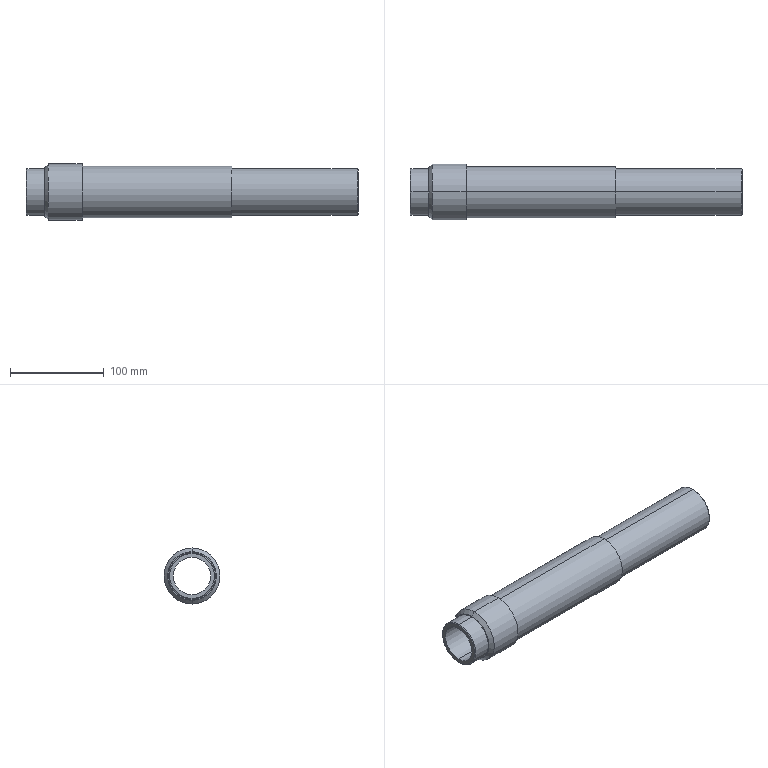Part | SolidWorks | features Chamfer 1, Fillet 1, Revolution 1 | 1 solid | 23 faces | box 355 x 60 x 60 mm | volume 349894 mm3 | cylinder 10 | plane 5 | cone 4 | torus 4 | commonest cylinder face diameters 50 x4 40 x2 55 x2 60 x2
STEP:
#1=CARTESIAN_POINT('',(354.,0.,20.));
#2=VERTEX_POINT('',#1);
#3=CARTESIAN_POINT('',(354.,0.,-20.));
#4=VERTEX_POINT('',#3);
#5=CARTESIAN_POINT('',(354.,0.,0.));
#6=DIRECTION('',(1.,0.,0.));
#7=DIRECTION('',(0.,0.,1.));
#8=AXIS2_PLACEMENT_3D('',#5,#6,#7);
#9=CIRCLE('',#8,20.);
#10=EDGE_CURVE('',#2,#4,#9,.T.);
#11=ORIENTED_EDGE('',*,*,#10,.F.);
#12=CARTESIAN_POINT('',(355.,0.,21.));
#13=VERTEX_POINT('',#12);
#14=CARTESIAN_POINT('',(355.,0.,21.));
#15=DIRECTION('',(0.7071,0.,0.7071));
#16=VECTOR('',#15,1000.);
#17=LINE('',#14,#16);
#18=EDGE_CURVE('',#2,#13,#17,.T.);
#19=ORIENTED_EDGE('',*,*,#18,.T.);
#20=CARTESIAN_POINT('',(355.,0.,-21.));
#21=VERTEX_POINT('',#20);
#22=CARTESIAN_POINT('',(355.,0.,0.));
#23=DIRECTION('',(-1.,0.,0.));
#24=DIRECTION('',(0.,0.,1.));
#25=AXIS2_PLACEMENT_3D('',#22,#23,#24);
#26=CIRCLE('',#25,21.);
#27=EDGE_CURVE('',#21,#13,#26,.T.);
#28=ORIENTED_EDGE('',*,*,#27,.F.);
#29=CARTESIAN_POINT('',(355.,0.,-21.));
#30=DIRECTION('',(0.7071,0.,-0.7071));
#31=VECTOR('',#30,1000.);
#32=LINE('',#29,#31);
#33=EDGE_CURVE('',#4,#21,#32,.T.);
#34=ORIENTED_EDGE('',*,*,#33,.F.);
#35=EDGE_LOOP('',(#11,#19,#28,#34));
#36=FACE_OUTER_BOUND('',#35,.T.);
#37=CARTESIAN_POINT('',(355.,0.,0.));
#38=DIRECTION('',(1.,0.,0.));
#39=DIRECTION('',(0.,0.,-1.));
#40=AXIS2_PLACEMENT_3D('',#37,#38,#39);
#41=CONICAL_SURFACE('',#40,21.,0.7854);
#42=ADVANCED_FACE('',(#36),#41,.F.);
#43=CARTESIAN_POINT('',(1.,0.,-25.));
#44=VERTEX_POINT('',#43);
#45=CARTESIAN_POINT('',(1.,0.,25.));
#46=VERTEX_POINT('',#45);
#47=CARTESIAN_POINT('',(1.,0.,0.));
#48=DIRECTION('',(1.,0.,0.));
#49=DIRECTION('',(0.,0.,1.));
#50=AXIS2_PLACEMENT_3D('',#47,#48,#49);
#51=CIRCLE('',#50,25.);
#52=EDGE_CURVE('',#44,#46,#51,.T.);
#53=ORIENTED_EDGE('',*,*,#52,.F.);
#54=CARTESIAN_POINT('',(0.,0.,-24.));
#55=VERTEX_POINT('',#54);
#56=CARTESIAN_POINT('',(1.,0.,-24.));
#57=DIRECTION('',(0.,1.,0.));
#58=DIRECTION('',(0.,0.,1.));
#59=AXIS2_PLACEMENT_3D('',#56,#57,#58);
#60=CIRCLE('',#59,1.);
#61=EDGE_CURVE('',#44,#55,#60,.T.);
#62=ORIENTED_EDGE('',*,*,#61,.T.);
#63=CARTESIAN_POINT('',(0.,0.,24.));
#64=VERTEX_POINT('',#63);
#65=CARTESIAN_POINT('',(0.,0.,0.));
#66=DIRECTION('',(-1.,0.,0.));
#67=DIRECTION('',(0.,0.,1.));
#68=AXIS2_PLACEMENT_3D('',#65,#66,#67);
#69=CIRCLE('',#68,24.);
#70=EDGE_CURVE('',#64,#55,#69,.T.);
#71=ORIENTED_EDGE('',*,*,#70,.F.);
#72=CARTESIAN_POINT('',(1.,0.,24.));
#73=DIRECTION('',(0.,-1.,0.));
#74=DIRECTION('',(0.,0.,-1.));
#75=AXIS2_PLACEMENT_3D('',#72,#73,#74);
#76=CIRCLE('',#75,1.);
#77=EDGE_CURVE('',#46,#64,#76,.T.);
#78=ORIENTED_EDGE('',*,*,#77,.F.);
#79=EDGE_LOOP('',(#53,#62,#71,#78));
#80=FACE_OUTER_BOUND('',#79,.T.);
#81=CARTESIAN_POINT('',(1.,0.,0.));
#82=DIRECTION('',(-1.,0.,0.));
#83=DIRECTION('',(0.,0.,1.));
#84=AXIS2_PLACEMENT_3D('',#81,#82,#83);
#85=TOROIDAL_SURFACE('',#84,24.,1.);
#86=ADVANCED_FACE('',(#80),#85,.T.);
#87=CARTESIAN_POINT('',(355.,0.,-24.));
#88=VERTEX_POINT('',#87);
#89=CARTESIAN_POINT('',(355.,0.,24.));
#90=VERTEX_POINT('',#89);
#91=CARTESIAN_POINT('',(355.,0.,0.));
#92=DIRECTION('',(1.,0.,0.));
#93=DIRECTION('',(0.,0.,1.));
#94=AXIS2_PLACEMENT_3D('',#91,#92,#93);
#95=CIRCLE('',#94,24.);
#96=EDGE_CURVE('',#88,#90,#95,.T.);
#97=ORIENTED_EDGE('',*,*,#96,.F.);
#98=CARTESIAN_POINT('',(354.,0.,-25.));
#99=VERTEX_POINT('',#98);
#100=CARTESIAN_POINT('',(354.,0.,-24.));
#101=DIRECTION('',(0.,1.,0.));
#102=DIRECTION('',(0.,0.,1.));
#103=AXIS2_PLACEMENT_3D('',#100,#101,#102);
#104=CIRCLE('',#103,1.);
#105=EDGE_CURVE('',#88,#99,#104,.T.);
#106=ORIENTED_EDGE('',*,*,#105,.T.);
#107=CARTESIAN_POINT('',(354.,0.,25.));
#108=VERTEX_POINT('',#107);
#109=CARTESIAN_POINT('',(354.,0.,0.));
#110=DIRECTION('',(-1.,0.,0.));
#111=DIRECTION('',(0.,0.,1.));
#112=AXIS2_PLACEMENT_3D('',#109,#110,#111);
#113=CIRCLE('',#112,25.);
#114=EDGE_CURVE('',#108,#99,#113,.T.);
#115=ORIENTED_EDGE('',*,*,#114,.F.);
#116=CARTESIAN_POINT('',(354.,0.,24.));
#117=DIRECTION('',(0.,-1.,0.));
#118=DIRECTION('',(0.,0.,-1.));
#119=AXIS2_PLACEMENT_3D('',#116,#117,#118);
#120=CIRCLE('',#119,1.);
#121=EDGE_CURVE('',#90,#108,#120,.T.);
#122=ORIENTED_EDGE('',*,*,#121,.F.);
#123=EDGE_LOOP('',(#97,#106,#115,#122));
#124=FACE_OUTER_BOUND('',#123,.T.);
#125=CARTESIAN_POINT('',(354.,0.,0.));
#126=DIRECTION('',(-1.,0.,0.));
#127=DIRECTION('',(0.,0.,1.));
#128=AXIS2_PLACEMENT_3D('',#125,#126,#127);
#129=TOROIDAL_SURFACE('',#128,24.,1.);
#130=ADVANCED_FACE('',(#124),#129,.T.);
#131=CARTESIAN_POINT('',(20.,0.,26.));
#132=VERTEX_POINT('',#131);
#133=CARTESIAN_POINT('',(20.,0.,-26.));
#134=VERTEX_POINT('',#133);
#135=CARTESIAN_POINT('',(20.,0.,0.));
#136=DIRECTION('',(-1.,0.,0.));
#137=DIRECTION('',(0.,0.,1.));
#138=AXIS2_PLACEMENT_3D('',#135,#136,#137);
#139=CIRCLE('',#138,26.);
#140=EDGE_CURVE('',#132,#134,#139,.T.);
#141=ORIENTED_EDGE('',*,*,#140,.F.);
#142=CARTESIAN_POINT('',(24.,0.,30.));
#143=VERTEX_POINT('',#142);
#144=CARTESIAN_POINT('',(20.,0.,26.));
#145=DIRECTION('',(0.7071,0.,0.7071));
#146=VECTOR('',#145,1000.);
#147=LINE('',#144,#146);
#148=EDGE_CURVE('',#132,#143,#147,.T.);
#149=ORIENTED_EDGE('',*,*,#148,.T.);
#150=CARTESIAN_POINT('',(24.,0.,-30.));
#151=VERTEX_POINT('',#150);
#152=CARTESIAN_POINT('',(24.,0.,0.));
#153=DIRECTION('',(-1.,0.,0.));
#154=DIRECTION('',(0.,0.,1.));
#155=AXIS2_PLACEMENT_3D('',#152,#153,#154);
#156=CIRCLE('',#155,30.);
#157=EDGE_CURVE('',#143,#151,#156,.T.);
#158=ORIENTED_EDGE('',*,*,#157,.T.);
#159=CARTESIAN_POINT('',(20.,0.,-26.));
#160=DIRECTION('',(0.7071,0.,-0.7071));
#161=VECTOR('',#160,1000.);
#162=LINE('',#159,#161);
#163=EDGE_CURVE('',#134,#151,#162,.T.);
#164=ORIENTED_EDGE('',*,*,#163,.F.);
#165=EDGE_LOOP('',(#141,#149,#158,#164));
#166=FACE_OUTER_BOUND('',#165,.T.);
#167=CARTESIAN_POINT('',(20.,0.,0.));
#168=DIRECTION('',(1.,0.,0.));
#169=DIRECTION('',(0.,0.,-1.));
#170=AXIS2_PLACEMENT_3D('',#167,#168,#169);
#171=CONICAL_SURFACE('',#170,26.,0.7854);
#172=ADVANCED_FACE('',(#166),#171,.T.);
#173=CARTESIAN_POINT('',(60.,0.,30.));
#174=VERTEX_POINT('',#173);
#175=CARTESIAN_POINT('',(60.,0.,-30.));
#176=VERTEX_POINT('',#175);
#177=CARTESIAN_POINT('',(60.,0.,0.));
#178=DIRECTION('',(-1.,0.,0.));
#179=DIRECTION('',(0.,0.,1.));
#180=AXIS2_PLACEMENT_3D('',#177,#178,#179);
#181=CIRCLE('',#180,30.);
#182=EDGE_CURVE('',#174,#176,#181,.T.);
#183=ORIENTED_EDGE('',*,*,#182,.T.);
#184=CARTESIAN_POINT('',(20.,0.,-30.));
#185=DIRECTION('',(-1.,0.,0.));
#186=VECTOR('',#185,1000.);
#187=LINE('',#184,#186);
#188=EDGE_CURVE('',#176,#151,#187,.T.);
#189=ORIENTED_EDGE('',*,*,#188,.T.);
#190=ORIENTED_EDGE('',*,*,#157,.F.);
#191=CARTESIAN_POINT('',(20.,0.,30.));
#192=DIRECTION('',(-1.,0.,0.));
#193=VECTOR('',#192,1000.);
#194=LINE('',#191,#193);
#195=EDGE_CURVE('',#174,#143,#194,.T.);
#196=ORIENTED_EDGE('',*,*,#195,.F.);
#197=EDGE_LOOP('',(#183,#189,#190,#196));
#198=FACE_OUTER_BOUND('',#197,.T.);
#199=CARTESIAN_POINT('',(20.,0.,0.));
#200=DIRECTION('',(-1.,0.,0.));
#201=DIRECTION('',(0.,0.,1.));
#202=AXIS2_PLACEMENT_3D('',#199,#200,#201);
#203=CYLINDRICAL_SURFACE('',#202,30.);
#204=ADVANCED_FACE('',(#198),#203,.T.);
#205=CARTESIAN_POINT('',(220.,0.,27.5));
#206=VERTEX_POINT('',#205);
#207=CARTESIAN_POINT('',(220.,0.,-27.5));
#208=VERTEX_POINT('',#207);
#209=CARTESIAN_POINT('',(220.,0.,0.));
#210=DIRECTION('',(-1.,0.,0.));
#211=DIRECTION('',(0.,0.,1.));
#212=AXIS2_PLACEMENT_3D('',#209,#210,#211);
#213=CIRCLE('',#212,27.5);
#214=EDGE_CURVE('',#206,#208,#213,.T.);
#215=ORIENTED_EDGE('',*,*,#214,.T.);
#216=CARTESIAN_POINT('',(60.,0.,-27.5));
#217=VERTEX_POINT('',#216);
#218=CARTESIAN_POINT('',(20.,0.,-27.5));
#219=DIRECTION('',(-1.,0.,0.));
#220=VECTOR('',#219,1000.);
#221=LINE('',#218,#220);
#222=EDGE_CURVE('',#208,#217,#221,.T.);
#223=ORIENTED_EDGE('',*,*,#222,.T.);
#224=CARTESIAN_POINT('',(60.,0.,27.5));
#225=VERTEX_POINT('',#224);
#226=CARTESIAN_POINT('',(60.,0.,0.));
#227=DIRECTION('',(-1.,0.,0.));
#228=DIRECTION('',(0.,0.,1.));
#229=AXIS2_PLACEMENT_3D('',#226,#227,#228);
#230=CIRCLE('',#229,27.5);
#231=EDGE_CURVE('',#225,#217,#230,.T.);
#232=ORIENTED_EDGE('',*,*,#231,.F.);
#233=CARTESIAN_POINT('',(20.,0.,27.5));
#234=DIRECTION('',(-1.,0.,0.));
#235=VECTOR('',#234,1000.);
#236=LINE('',#233,#235);
#237=EDGE_CURVE('',#206,#225,#236,.T.);
#238=ORIENTED_EDGE('',*,*,#237,.F.);
#239=EDGE_LOOP('',(#215,#223,#232,#238));
#240=FACE_OUTER_BOUND('',#239,.T.);
#241=CARTESIAN_POINT('',(20.,0.,0.));
#242=DIRECTION('',(-1.,0.,0.));
#243=DIRECTION('',(0.,0.,1.));
#244=AXIS2_PLACEMENT_3D('',#241,#242,#243);
#245=CYLINDRICAL_SURFACE('',#244,27.5);
#246=ADVANCED_FACE('',(#240),#245,.T.);
#247=ORIENTED_EDGE('',*,*,#114,.T.);
#248=CARTESIAN_POINT('',(220.,0.,-25.));
#249=VERTEX_POINT('',#248);
#250=CARTESIAN_POINT('',(20.,0.,-25.));
#251=DIRECTION('',(-1.,0.,0.));
#252=VECTOR('',#251,1000.);
#253=LINE('',#250,#252);
#254=EDGE_CURVE('',#99,#249,#253,.T.);
#255=ORIENTED_EDGE('',*,*,#254,.T.);
#256=CARTESIAN_POINT('',(220.,0.,25.));
#257=VERTEX_POINT('',#256);
#258=CARTESIAN_POINT('',(220.,0.,0.));
#259=DIRECTION('',(-1.,0.,0.));
#260=DIRECTION('',(0.,0.,1.));
#261=AXIS2_PLACEMENT_3D('',#258,#259,#260);
#262=CIRCLE('',#261,25.);
#263=EDGE_CURVE('',#257,#249,#262,.T.);
#264=ORIENTED_EDGE('',*,*,#263,.F.);
#265=CARTESIAN_POINT('',(20.,0.,25.));
#266=DIRECTION('',(-1.,0.,0.));
#267=VECTOR('',#266,1000.);
#268=LINE('',#265,#267);
#269=EDGE_CURVE('',#108,#257,#268,.T.);
#270=ORIENTED_EDGE('',*,*,#269,.F.);
#271=EDGE_LOOP('',(#247,#255,#264,#270));
#272=FACE_OUTER_BOUND('',#271,.T.);
#273=CARTESIAN_POINT('',(20.,0.,0.));
#274=DIRECTION('',(-1.,0.,0.));
#275=DIRECTION('',(0.,0.,1.));
#276=AXIS2_PLACEMENT_3D('',#273,#274,#275);
#277=CYLINDRICAL_SURFACE('',#276,25.);
#278=ADVANCED_FACE('',(#272),#277,.T.);
#279=ORIENTED_EDGE('',*,*,#10,.T.);
#280=CARTESIAN_POINT('',(0.,0.,-20.));
#281=VERTEX_POINT('',#280);
#282=CARTESIAN_POINT('',(20.,0.,-20.));
#283=DIRECTION('',(-1.,0.,0.));
#284=VECTOR('',#283,1000.);
#285=LINE('',#282,#284);
#286=EDGE_CURVE('',#4,#281,#285,.T.);
#287=ORIENTED_EDGE('',*,*,#286,.T.);
#288=CARTESIAN_POINT('',(0.,0.,20.));
#289=VERTEX_POINT('',#288);
#290=CARTESIAN_POINT('',(0.,0.,0.));
#291=DIRECTION('',(-1.,0.,0.));
#292=DIRECTION('',(0.,0.,1.));
#293=AXIS2_PLACEMENT_3D('',#290,#291,#292);
#294=CIRCLE('',#293,20.);
#295=EDGE_CURVE('',#281,#289,#294,.T.);
#296=ORIENTED_EDGE('',*,*,#295,.T.);
#297=CARTESIAN_POINT('',(20.,0.,20.));
#298=DIRECTION('',(-1.,0.,0.));
#299=VECTOR('',#298,1000.);
#300=LINE('',#297,#299);
#301=EDGE_CURVE('',#2,#289,#300,.T.);
#302=ORIENTED_EDGE('',*,*,#301,.F.);
#303=EDGE_LOOP('',(#279,#287,#296,#302));
#304=FACE_OUTER_BOUND('',#303,.T.);
#305=CARTESIAN_POINT('',(20.,0.,0.));
#306=DIRECTION('',(-1.,0.,0.));
#307=DIRECTION('',(0.,0.,1.));
#308=AXIS2_PLACEMENT_3D('',#305,#306,#307);
#309=CYLINDRICAL_SURFACE('',#308,20.);
#310=ADVANCED_FACE('',(#304),#309,.F.);
#311=CARTESIAN_POINT('',(20.,0.,25.));
#312=VERTEX_POINT('',#311);
#313=CARTESIAN_POINT('',(20.,0.,-25.));
#314=VERTEX_POINT('',#313);
#315=CARTESIAN_POINT('',(20.,0.,0.));
#316=DIRECTION('',(-1.,0.,0.));
#317=DIRECTION('',(0.,0.,1.));
#318=AXIS2_PLACEMENT_3D('',#315,#316,#317);
#319=CIRCLE('',#318,25.);
#320=EDGE_CURVE('',#312,#314,#319,.T.);
#321=ORIENTED_EDGE('',*,*,#320,.T.);
#322=CARTESIAN_POINT('',(20.,0.,-25.));
#323=DIRECTION('',(-1.,0.,0.));
#324=VECTOR('',#323,1000.);
#325=LINE('',#322,#324);
#326=EDGE_CURVE('',#314,#44,#325,.T.);
#327=ORIENTED_EDGE('',*,*,#326,.T.);
#328=ORIENTED_EDGE('',*,*,#52,.T.);
#329=CARTESIAN_POINT('',(20.,0.,25.));
#330=DIRECTION('',(-1.,0.,0.));
#331=VECTOR('',#330,1000.);
#332=LINE('',#329,#331);
#333=EDGE_CURVE('',#312,#46,#332,.T.);
#334=ORIENTED_EDGE('',*,*,#333,.F.);
#335=EDGE_LOOP('',(#321,#327,#328,#334));
#336=FACE_OUTER_BOUND('',#335,.T.);
#337=CARTESIAN_POINT('',(20.,0.,0.));
#338=DIRECTION('',(-1.,0.,0.));
#339=DIRECTION('',(0.,0.,1.));
#340=AXIS2_PLACEMENT_3D('',#337,#338,#339);
#341=CYLINDRICAL_SURFACE('',#340,25.);
#342=ADVANCED_FACE('',(#336),#341,.T.);
#343=ORIENTED_EDGE('',*,*,#326,.F.);
#344=CARTESIAN_POINT('',(20.,0.,0.));
#345=DIRECTION('',(-1.,0.,0.));
#346=DIRECTION('',(0.,0.,1.));
#347=AXIS2_PLACEMENT_3D('',#344,#345,#346);
#348=CIRCLE('',#347,25.);
#349=EDGE_CURVE('',#314,#312,#348,.T.);
#350=ORIENTED_EDGE('',*,*,#349,.T.);
#351=ORIENTED_EDGE('',*,*,#333,.T.);
#352=CARTESIAN_POINT('',(1.,0.,0.));
#353=DIRECTION('',(1.,0.,0.));
#354=DIRECTION('',(0.,0.,1.));
#355=AXIS2_PLACEMENT_3D('',#352,#353,#354);
#356=CIRCLE('',#355,25.);
#357=EDGE_CURVE('',#46,#44,#356,.T.);
#358=ORIENTED_EDGE('',*,*,#357,.T.);
#359=EDGE_LOOP('',(#343,#350,#351,#358));
#360=FACE_OUTER_BOUND('',#359,.T.);
#361=CARTESIAN_POINT('',(20.,0.,0.));
#362=DIRECTION('',(-1.,0.,0.));
#363=DIRECTION('',(0.,0.,1.));
#364=AXIS2_PLACEMENT_3D('',#361,#362,#363);
#365=CYLINDRICAL_SURFACE('',#364,25.);
#366=ADVANCED_FACE('',(#360),#365,.T.);
#367=ORIENTED_EDGE('',*,*,#70,.T.);
#368=CARTESIAN_POINT('',(0.,0.,0.));
#369=DIRECTION('',(-1.,0.,0.));
#370=DIRECTION('',(0.,0.,1.));
#371=AXIS2_PLACEMENT_3D('',#368,#369,#370);
#372=CIRCLE('',#371,24.);
#373=EDGE_CURVE('',#55,#64,#372,.T.);
#374=ORIENTED_EDGE('',*,*,#373,.T.);
#375=EDGE_LOOP('',(#367,#374));
#376=FACE_OUTER_BOUND('',#375,.T.);
#377=CARTESIAN_POINT('',(0.,0.,0.));
#378=DIRECTION('',(-1.,0.,0.));
#379=DIRECTION('',(0.,0.,1.));
#380=AXIS2_PLACEMENT_3D('',#377,#378,#379);
#381=CIRCLE('',#380,20.);
#382=EDGE_CURVE('',#289,#281,#381,.T.);
#383=ORIENTED_EDGE('',*,*,#382,.F.);
#384=ORIENTED_EDGE('',*,*,#295,.F.);
#385=EDGE_LOOP('',(#383,#384));
#386=FACE_BOUND('',#385,.T.);
#387=CARTESIAN_POINT('',(0.,0.,0.));
#388=DIRECTION('',(-1.,0.,0.));
#389=DIRECTION('',(0.,0.,1.));
#390=AXIS2_PLACEMENT_3D('',#387,#388,#389);
#391=PLANE('',#390);
#392=ADVANCED_FACE('',(#376,#386),#391,.T.);
#393=ORIENTED_EDGE('',*,*,#286,.F.);
#394=CARTESIAN_POINT('',(354.,0.,0.));
#395=DIRECTION('',(1.,0.,0.));
#396=DIRECTION('',(0.,0.,1.));
#397=AXIS2_PLACEMENT_3D('',#394,#395,#396);
#398=CIRCLE('',#397,20.);
#399=EDGE_CURVE('',#4,#2,#398,.T.);
#400=ORIENTED_EDGE('',*,*,#399,.T.);
#401=ORIENTED_EDGE('',*,*,#301,.T.);
#402=ORIENTED_EDGE('',*,*,#382,.T.);
#403=EDGE_LOOP('',(#393,#400,#401,#402));
#404=FACE_OUTER_BOUND('',#403,.T.);
#405=CARTESIAN_POINT('',(20.,0.,0.));
#406=DIRECTION('',(-1.,0.,0.));
#407=DIRECTION('',(0.,0.,1.));
#408=AXIS2_PLACEMENT_3D('',#405,#406,#407);
#409=CYLINDRICAL_SURFACE('',#408,20.);
#410=ADVANCED_FACE('',(#404),#409,.F.);
#411=ORIENTED_EDGE('',*,*,#27,.T.);
#412=CARTESIAN_POINT('',(355.,0.,0.));
#413=DIRECTION('',(-1.,0.,0.));
#414=DIRECTION('',(0.,0.,1.));
#415=AXIS2_PLACEMENT_3D('',#412,#413,#414);
#416=CIRCLE('',#415,21.);
#417=EDGE_CURVE('',#13,#21,#416,.T.);
#418=ORIENTED_EDGE('',*,*,#417,.T.);
#419=EDGE_LOOP('',(#411,#418));
#420=FACE_BOUND('',#419,.T.);
#421=CARTESIAN_POINT('',(355.,0.,0.));
#422=DIRECTION('',(1.,0.,0.));
#423=DIRECTION('',(0.,0.,1.));
#424=AXIS2_PLACEMENT_3D('',#421,#422,#423);
#425=CIRCLE('',#424,24.);
#426=EDGE_CURVE('',#90,#88,#425,.T.);
#427=ORIENTED_EDGE('',*,*,#426,.T.);
#428=ORIENTED_EDGE('',*,*,#96,.T.);
#429=EDGE_LOOP('',(#427,#428));
#430=FACE_OUTER_BOUND('',#429,.T.);
#431=CARTESIAN_POINT('',(355.,0.,0.));
#432=DIRECTION('',(-1.,0.,0.));
#433=DIRECTION('',(0.,0.,1.));
#434=AXIS2_PLACEMENT_3D('',#431,#432,#433);
#435=PLANE('',#434);
#436=ADVANCED_FACE('',(#420,#430),#435,.F.);
#437=ORIENTED_EDGE('',*,*,#254,.F.);
#438=CARTESIAN_POINT('',(354.,0.,0.));
#439=DIRECTION('',(-1.,0.,0.));
#440=DIRECTION('',(0.,0.,1.));
#441=AXIS2_PLACEMENT_3D('',#438,#439,#440);
#442=CIRCLE('',#441,25.);
#443=EDGE_CURVE('',#99,#108,#442,.T.);
#444=ORIENTED_EDGE('',*,*,#443,.T.);
#445=ORIENTED_EDGE('',*,*,#269,.T.);
#446=CARTESIAN_POINT('',(220.,0.,0.));
#447=DIRECTION('',(-1.,0.,0.));
#448=DIRECTION('',(0.,0.,1.));
#449=AXIS2_PLACEMENT_3D('',#446,#447,#448);
#450=CIRCLE('',#449,25.);
#451=EDGE_CURVE('',#249,#257,#450,.T.);
#452=ORIENTED_EDGE('',*,*,#451,.F.);
#453=EDGE_LOOP('',(#437,#444,#445,#452));
#454=FACE_OUTER_BOUND('',#453,.T.);
#455=CARTESIAN_POINT('',(20.,0.,0.));
#456=DIRECTION('',(-1.,0.,0.));
#457=DIRECTION('',(0.,0.,1.));
#458=AXIS2_PLACEMENT_3D('',#455,#456,#457);
#459=CYLINDRICAL_SURFACE('',#458,25.);
#460=ADVANCED_FACE('',(#454),#459,.T.);
#461=ORIENTED_EDGE('',*,*,#214,.F.);
#462=CARTESIAN_POINT('',(220.,0.,0.));
#463=DIRECTION('',(-1.,0.,0.));
#464=DIRECTION('',(0.,0.,1.));
#465=AXIS2_PLACEMENT_3D('',#462,#463,#464);
#466=CIRCLE('',#465,27.5);
#467=EDGE_CURVE('',#208,#206,#466,.T.);
#468=ORIENTED_EDGE('',*,*,#467,.F.);
#469=EDGE_LOOP('',(#461,#468));
#470=FACE_OUTER_BOUND('',#469,.T.);
#471=ORIENTED_EDGE('',*,*,#263,.T.);
#472=ORIENTED_EDGE('',*,*,#451,.T.);
#473=EDGE_LOOP('',(#471,#472));
#474=FACE_BOUND('',#473,.T.);
#475=CARTESIAN_POINT('',(220.,0.,0.));
#476=DIRECTION('',(-1.,0.,0.));
#477=DIRECTION('',(0.,0.,1.));
#478=AXIS2_PLACEMENT_3D('',#475,#476,#477);
#479=PLANE('',#478);
#480=ADVANCED_FACE('',(#470,#474),#479,.F.);
#481=ORIENTED_EDGE('',*,*,#222,.F.);
#482=ORIENTED_EDGE('',*,*,#467,.T.);
#483=ORIENTED_EDGE('',*,*,#237,.T.);
#484=CARTESIAN_POINT('',(60.,0.,0.));
#485=DIRECTION('',(-1.,0.,0.));
#486=DIRECTION('',(0.,0.,1.));
#487=AXIS2_PLACEMENT_3D('',#484,#485,#486);
#488=CIRCLE('',#487,27.5);
#489=EDGE_CURVE('',#217,#225,#488,.T.);
#490=ORIENTED_EDGE('',*,*,#489,.F.);
#491=EDGE_LOOP('',(#481,#482,#483,#490));
#492=FACE_OUTER_BOUND('',#491,.T.);
#493=CARTESIAN_POINT('',(20.,0.,0.));
#494=DIRECTION('',(-1.,0.,0.));
#495=DIRECTION('',(0.,0.,1.));
#496=AXIS2_PLACEMENT_3D('',#493,#494,#495);
#497=CYLINDRICAL_SURFACE('',#496,27.5);
#498=ADVANCED_FACE('',(#492),#497,.T.);
#499=ORIENTED_EDGE('',*,*,#182,.F.);
#500=CARTESIAN_POINT('',(60.,0.,0.));
#501=DIRECTION('',(-1.,0.,0.));
#502=DIRECTION('',(0.,0.,1.));
#503=AXIS2_PLACEMENT_3D('',#500,#501,#502);
#504=CIRCLE('',#503,30.);
#505=EDGE_CURVE('',#176,#174,#504,.T.);
#506=ORIENTED_EDGE('',*,*,#505,.F.);
#507=EDGE_LOOP('',(#499,#506));
#508=FACE_OUTER_BOUND('',#507,.T.);
#509=ORIENTED_EDGE('',*,*,#231,.T.);
#510=ORIENTED_EDGE('',*,*,#489,.T.);
#511=EDGE_LOOP('',(#509,#510));
#512=FACE_BOUND('',#511,.T.);
#513=CARTESIAN_POINT('',(60.,0.,0.));
#514=DIRECTION('',(-1.,0.,0.));
#515=DIRECTION('',(0.,0.,1.));
#516=AXIS2_PLACEMENT_3D('',#513,#514,#515);
#517=PLANE('',#516);
#518=ADVANCED_FACE('',(#508,#512),#517,.F.);
#519=ORIENTED_EDGE('',*,*,#188,.F.);
#520=ORIENTED_EDGE('',*,*,#505,.T.);
#521=ORIENTED_EDGE('',*,*,#195,.T.);
#522=CARTESIAN_POINT('',(24.,0.,0.));
#523=DIRECTION('',(-1.,0.,0.));
#524=DIRECTION('',(0.,0.,1.));
#525=AXIS2_PLACEMENT_3D('',#522,#523,#524);
#526=CIRCLE('',#525,30.);
#527=EDGE_CURVE('',#151,#143,#526,.T.);
#528=ORIENTED_EDGE('',*,*,#527,.F.);
#529=EDGE_LOOP('',(#519,#520,#521,#528));
#530=FACE_OUTER_BOUND('',#529,.T.);
#531=CARTESIAN_POINT('',(20.,0.,0.));
#532=DIRECTION('',(-1.,0.,0.));
#533=DIRECTION('',(0.,0.,1.));
#534=AXIS2_PLACEMENT_3D('',#531,#532,#533);
#535=CYLINDRICAL_SURFACE('',#534,30.);
#536=ADVANCED_FACE('',(#530),#535,.T.);
#537=ORIENTED_EDGE('',*,*,#148,.F.);
#538=CARTESIAN_POINT('',(20.,0.,0.));
#539=DIRECTION('',(-1.,0.,0.));
#540=DIRECTION('',(0.,0.,1.));
#541=AXIS2_PLACEMENT_3D('',#538,#539,#540);
#542=CIRCLE('',#541,26.);
#543=EDGE_CURVE('',#134,#132,#542,.T.);
#544=ORIENTED_EDGE('',*,*,#543,.F.);
#545=ORIENTED_EDGE('',*,*,#163,.T.);
#546=ORIENTED_EDGE('',*,*,#527,.T.);
#547=EDGE_LOOP('',(#537,#544,#545,#546));
#548=FACE_OUTER_BOUND('',#547,.T.);
#549=CARTESIAN_POINT('',(20.,0.,0.));
#550=DIRECTION('',(1.,0.,0.));
#551=DIRECTION('',(0.,0.,-1.));
#552=AXIS2_PLACEMENT_3D('',#549,#550,#551);
#553=CONICAL_SURFACE('',#552,26.,0.7854);
#554=ADVANCED_FACE('',(#548),#553,.T.);
#555=ORIENTED_EDGE('',*,*,#543,.T.);
#556=ORIENTED_EDGE('',*,*,#140,.T.);
#557=EDGE_LOOP('',(#555,#556));
#558=FACE_OUTER_BOUND('',#557,.T.);
#559=ORIENTED_EDGE('',*,*,#320,.F.);
#560=ORIENTED_EDGE('',*,*,#349,.F.);
#561=EDGE_LOOP('',(#559,#560));
#562=FACE_BOUND('',#561,.T.);
#563=CARTESIAN_POINT('',(20.,0.,0.));
#564=DIRECTION('',(-1.,0.,0.));
#565=DIRECTION('',(0.,0.,1.));
#566=AXIS2_PLACEMENT_3D('',#563,#564,#565);
#567=PLANE('',#566);
#568=ADVANCED_FACE('',(#558,#562),#567,.T.);
#569=ORIENTED_EDGE('',*,*,#105,.F.);
#570=ORIENTED_EDGE('',*,*,#426,.F.);
#571=ORIENTED_EDGE('',*,*,#121,.T.);
#572=ORIENTED_EDGE('',*,*,#443,.F.);
#573=EDGE_LOOP('',(#569,#570,#571,#572));
#574=FACE_OUTER_BOUND('',#573,.T.);
#575=CARTESIAN_POINT('',(354.,0.,0.));
#576=DIRECTION('',(-1.,0.,0.));
#577=DIRECTION('',(0.,0.,1.));
#578=AXIS2_PLACEMENT_3D('',#575,#576,#577);
#579=TOROIDAL_SURFACE('',#578,24.,1.);
#580=ADVANCED_FACE('',(#574),#579,.T.);
#581=ORIENTED_EDGE('',*,*,#61,.F.);
#582=ORIENTED_EDGE('',*,*,#357,.F.);
#583=ORIENTED_EDGE('',*,*,#77,.T.);
#584=ORIENTED_EDGE('',*,*,#373,.F.);
#585=EDGE_LOOP('',(#581,#582,#583,#584));
#586=FACE_OUTER_BOUND('',#585,.T.);
#587=CARTESIAN_POINT('',(1.,0.,0.));
#588=DIRECTION('',(-1.,0.,0.));
#589=DIRECTION('',(0.,0.,1.));
#590=AXIS2_PLACEMENT_3D('',#587,#588,#589);
#591=TOROIDAL_SURFACE('',#590,24.,1.);
#592=ADVANCED_FACE('',(#586),#591,.T.);
#593=ORIENTED_EDGE('',*,*,#18,.F.);
#594=ORIENTED_EDGE('',*,*,#399,.F.);
#595=ORIENTED_EDGE('',*,*,#33,.T.);
#596=ORIENTED_EDGE('',*,*,#417,.F.);
#597=EDGE_LOOP('',(#593,#594,#595,#596));
#598=FACE_OUTER_BOUND('',#597,.T.);
#599=CARTESIAN_POINT('',(355.,0.,0.));
#600=DIRECTION('',(1.,0.,0.));
#601=DIRECTION('',(0.,0.,-1.));
#602=AXIS2_PLACEMENT_3D('',#599,#600,#601);
#603=CONICAL_SURFACE('',#602,21.,0.7854);
#604=ADVANCED_FACE('',(#598),#603,.F.);
#605=CLOSED_SHELL('',(#42,#86,#130,#172,#204,#246,#278,#310,#342,#366,#392,#410,#436,#460,#480,#498,#518,#536,#554,#568,#580,#592,#604));
#606=MANIFOLD_SOLID_BREP('',#605);
#607=CARTESIAN_POINT('',(0.,0.,0.));
#608=DIRECTION('',(0.,0.,1.));
#609=DIRECTION('',(1.,0.,0.));
#610=AXIS2_PLACEMENT_3D('',#607,#608,#609);
#611=(LENGTH_UNIT()NAMED_UNIT(*)SI_UNIT(.MILLI.,.METRE.));
#612=UNCERTAINTY_MEASURE_WITH_UNIT(LENGTH_MEASURE(0.00001),#611,'','');
#613=(NAMED_UNIT(*)PLANE_ANGLE_UNIT()SI_UNIT($,.RADIAN.));
#614=(NAMED_UNIT(*)SI_UNIT($,.STERADIAN.)SOLID_ANGLE_UNIT());
#615=(GEOMETRIC_REPRESENTATION_CONTEXT(3)GLOBAL_UNCERTAINTY_ASSIGNED_CONTEXT((#612))GLOBAL_UNIT_ASSIGNED_CONTEXT((#611,#613,#614))REPRESENTATION_CONTEXT('',''));
#616=ADVANCED_BREP_SHAPE_REPRESENTATION('',(#606,#610),#615);